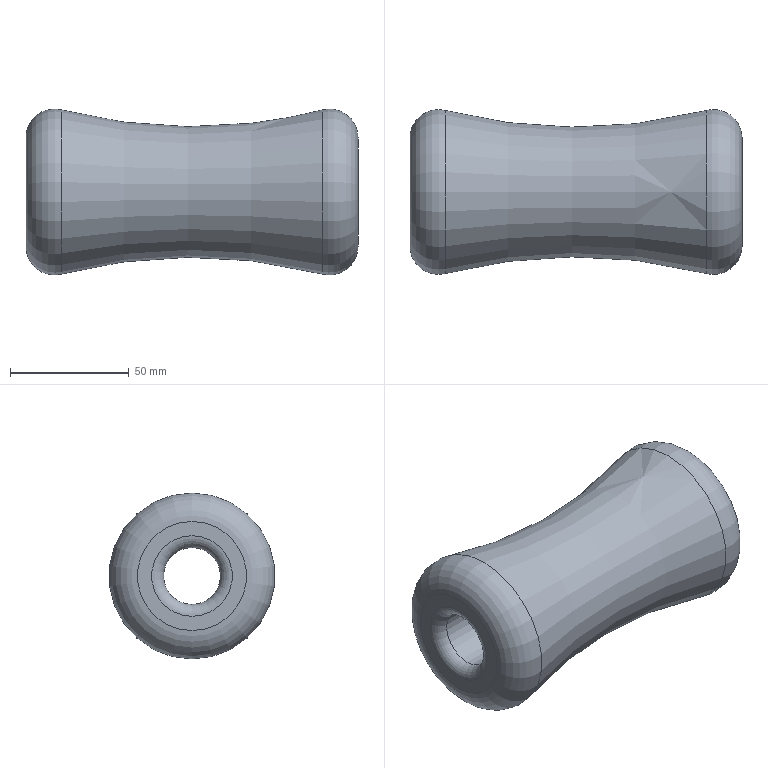Part | STEP file | 6101402W | 1 solid | 8 faces | box 140 x 70 x 70 mm | volume 348651 mm3 | torus 5 | plane 2 | cylinder 1 | commonest cylinder face diameters 24 x1
STEP:
#1=CARTESIAN_POINT('',(0.,0.,0.));
#2=DIRECTION('',(0.,0.,1.));
#3=DIRECTION('',(1.,0.,0.));
#4=AXIS2_PLACEMENT_3D('',#1,#2,#3);
#5=CARTESIAN_POINT('',(70.,0.,17.));
#6=VERTEX_POINT('',#5);
#7=CARTESIAN_POINT('',(70.,0.,0.));
#8=DIRECTION('',(-1.,0.,0.));
#9=DIRECTION('',(0.,0.,1.));
#10=AXIS2_PLACEMENT_3D('',#7,#8,#9);
#11=CIRCLE('',#10,17.);
#12=CARTESIAN_POINT('',(65.,0.,0.));
#13=DIRECTION('',(-1.,0.,0.));
#14=DIRECTION('',(0.,0.,1.));
#15=AXIS2_PLACEMENT_3D('',#12,#13,#14);
#16=TOROIDAL_SURFACE('',#15,17.,5.);
#17=CARTESIAN_POINT('',(0.,4.712));
#18=DIRECTION('',(1.,0.));
#19=VECTOR('',#18,1.);
#20=LINE('',#17,#19);
#21=(GEOMETRIC_REPRESENTATION_CONTEXT(2)PARAMETRIC_REPRESENTATION_CONTEXT()REPRESENTATION_CONTEXT('',''));
#22=DEFINITIONAL_REPRESENTATION('',(#20),#21);
#23=PCURVE('',#16,#22);
#24=CARTESIAN_POINT('',(70.,23.,0.));
#25=DIRECTION('',(-1.,0.,0.));
#26=DIRECTION('',(0.,0.,1.));
#27=AXIS2_PLACEMENT_3D('',#24,#25,#26);
#28=PLANE('',#27);
#29=CARTESIAN_POINT('',(0.,-23.));
#30=DIRECTION('',(1.,0.));
#31=AXIS2_PLACEMENT_2D('',#29,#30);
#32=CIRCLE('',#31,17.);
#33=(GEOMETRIC_REPRESENTATION_CONTEXT(2)PARAMETRIC_REPRESENTATION_CONTEXT()REPRESENTATION_CONTEXT('',''));
#34=DEFINITIONAL_REPRESENTATION('',(#32),#33);
#35=PCURVE('',#28,#34);
#36=SURFACE_CURVE('',#11,(#23,#35),.PCURVE_S1.);
#37=EDGE_CURVE('',#6,#6,#36,.T.);
#38=ORIENTED_EDGE('',*,*,#37,.F.);
#39=CARTESIAN_POINT('',(65.,0.,12.));
#40=VERTEX_POINT('',#39);
#41=CARTESIAN_POINT('',(65.,0.,12.));
#42=CARTESIAN_POINT('',(66.337,0.,12.));
#43=CARTESIAN_POINT('',(67.639,0.,12.425));
#44=CARTESIAN_POINT('',(68.76,0.,13.24));
#45=CARTESIAN_POINT('',(69.575,0.,14.361));
#46=CARTESIAN_POINT('',(70.,0.,15.663));
#47=CARTESIAN_POINT('',(70.,0.,17.));
#48=(BOUNDED_CURVE()B_SPLINE_CURVE(6,(#41,#42,#43,#44,#45,#46,#47),.UNSPECIFIED.,.F.,.F.)B_SPLINE_CURVE_WITH_KNOTS((7,7),(3.142,4.712),.PIECEWISE_BEZIER_KNOTS.)CURVE()GEOMETRIC_REPRESENTATION_ITEM()RATIONAL_B_SPLINE_CURVE((1.031,1.01,0.9979,0.994,0.9979,1.01,1.031))REPRESENTATION_ITEM(''));
#49=CARTESIAN_POINT('',(0.,0.));
#50=DIRECTION('',(0.,1.));
#51=VECTOR('',#50,1.);
#52=LINE('',#49,#51);
#53=(GEOMETRIC_REPRESENTATION_CONTEXT(2)PARAMETRIC_REPRESENTATION_CONTEXT()REPRESENTATION_CONTEXT('',''));
#54=DEFINITIONAL_REPRESENTATION('',(#52),#53);
#55=PCURVE('',#16,#54);
#56=CARTESIAN_POINT('',(6.283,0.));
#57=DIRECTION('',(0.,1.));
#58=VECTOR('',#57,1.);
#59=LINE('',#56,#58);
#60=(GEOMETRIC_REPRESENTATION_CONTEXT(2)PARAMETRIC_REPRESENTATION_CONTEXT()REPRESENTATION_CONTEXT('',''));
#61=DEFINITIONAL_REPRESENTATION('',(#59),#60);
#62=PCURVE('',#16,#61);
#63=SEAM_CURVE('',#48,(#55,#62),.PCURVE_S1.);
#64=EDGE_CURVE('',#40,#6,#63,.T.);
#65=ORIENTED_EDGE('',*,*,#64,.F.);
#66=CARTESIAN_POINT('',(65.,0.,0.));
#67=DIRECTION('',(-1.,0.,0.));
#68=DIRECTION('',(0.,0.,1.));
#69=AXIS2_PLACEMENT_3D('',#66,#67,#68);
#70=CIRCLE('',#69,12.);
#71=CARTESIAN_POINT('',(0.,3.142));
#72=DIRECTION('',(1.,0.));
#73=VECTOR('',#72,1.);
#74=LINE('',#71,#73);
#75=(GEOMETRIC_REPRESENTATION_CONTEXT(2)PARAMETRIC_REPRESENTATION_CONTEXT()REPRESENTATION_CONTEXT('',''));
#76=DEFINITIONAL_REPRESENTATION('',(#74),#75);
#77=PCURVE('',#16,#76);
#78=CARTESIAN_POINT('',(-73.428,0.,0.));
#79=DIRECTION('',(-1.,0.,0.));
#80=DIRECTION('',(0.,0.,1.));
#81=AXIS2_PLACEMENT_3D('',#78,#79,#80);
#82=CYLINDRICAL_SURFACE('',#81,12.);
#83=CARTESIAN_POINT('',(0.,-138.428));
#84=DIRECTION('',(1.,0.));
#85=VECTOR('',#84,1.);
#86=LINE('',#83,#85);
#87=(GEOMETRIC_REPRESENTATION_CONTEXT(2)PARAMETRIC_REPRESENTATION_CONTEXT()REPRESENTATION_CONTEXT('',''));
#88=DEFINITIONAL_REPRESENTATION('',(#86),#87);
#89=PCURVE('',#82,#88);
#90=SURFACE_CURVE('',#70,(#77,#89),.PCURVE_S1.);
#91=EDGE_CURVE('',#40,#40,#90,.T.);
#92=ORIENTED_EDGE('',*,*,#91,.T.);
#93=ORIENTED_EDGE('',*,*,#64,.T.);
#94=EDGE_LOOP('',(#38,#65,#92,#93));
#95=FACE_BOUND('',#94,.T.);
#96=ADVANCED_FACE('',(#95),#16,.T.);
#97=CARTESIAN_POINT('',(70.,0.,23.));
#98=VERTEX_POINT('',#97);
#99=CARTESIAN_POINT('',(70.,0.,0.));
#100=DIRECTION('',(-1.,0.,0.));
#101=DIRECTION('',(0.,0.,1.));
#102=AXIS2_PLACEMENT_3D('',#99,#100,#101);
#103=CIRCLE('',#102,23.);
#104=CARTESIAN_POINT('',(0.,-23.));
#105=DIRECTION('',(1.,0.));
#106=AXIS2_PLACEMENT_2D('',#104,#105);
#107=CIRCLE('',#106,23.);
#108=(GEOMETRIC_REPRESENTATION_CONTEXT(2)PARAMETRIC_REPRESENTATION_CONTEXT()REPRESENTATION_CONTEXT('',''));
#109=DEFINITIONAL_REPRESENTATION('',(#107),#108);
#110=PCURVE('',#28,#109);
#111=CARTESIAN_POINT('',(58.,0.,0.));
#112=DIRECTION('',(-1.,0.,0.));
#113=DIRECTION('',(0.,0.,1.));
#114=AXIS2_PLACEMENT_3D('',#111,#112,#113);
#115=TOROIDAL_SURFACE('',#114,23.,12.);
#116=CARTESIAN_POINT('',(0.,4.712));
#117=DIRECTION('',(1.,0.));
#118=VECTOR('',#117,1.);
#119=LINE('',#116,#118);
#120=(GEOMETRIC_REPRESENTATION_CONTEXT(2)PARAMETRIC_REPRESENTATION_CONTEXT()REPRESENTATION_CONTEXT('',''));
#121=DEFINITIONAL_REPRESENTATION('',(#119),#120);
#122=PCURVE('',#115,#121);
#123=SURFACE_CURVE('',#103,(#110,#122),.PCURVE_S1.);
#124=EDGE_CURVE('',#98,#98,#123,.T.);
#125=ORIENTED_EDGE('',*,*,#124,.F.);
#126=EDGE_LOOP('',(#125));
#127=FACE_BOUND('',#126,.T.);
#128=ORIENTED_EDGE('',*,*,#37,.T.);
#129=EDGE_LOOP('',(#128));
#130=FACE_BOUND('',#129,.T.);
#131=ADVANCED_FACE('',(#127,#130),#28,.F.);
#132=CARTESIAN_POINT('',(54.963,0.,34.609));
#133=VERTEX_POINT('',#132);
#134=CARTESIAN_POINT('',(54.963,0.,0.));
#135=DIRECTION('',(-1.,0.,0.));
#136=DIRECTION('',(0.,0.,1.));
#137=AXIS2_PLACEMENT_3D('',#134,#135,#136);
#138=CIRCLE('',#137,34.609);
#139=CARTESIAN_POINT('',(0.,6.539));
#140=DIRECTION('',(1.,0.));
#141=VECTOR('',#140,1.);
#142=LINE('',#139,#141);
#143=(GEOMETRIC_REPRESENTATION_CONTEXT(2)PARAMETRIC_REPRESENTATION_CONTEXT()REPRESENTATION_CONTEXT('',''));
#144=DEFINITIONAL_REPRESENTATION('',(#142),#143);
#145=PCURVE('',#115,#144);
#146=CARTESIAN_POINT('',(0.,0.,0.));
#147=DIRECTION('',(-1.,0.,0.));
#148=DIRECTION('',(0.,0.,1.));
#149=AXIS2_PLACEMENT_3D('',#146,#147,#148);
#150=TOROIDAL_SURFACE('',#149,244.698,217.16);
#151=CARTESIAN_POINT('',(0.,3.397));
#152=DIRECTION('',(1.,0.));
#153=VECTOR('',#152,1.);
#154=LINE('',#151,#153);
#155=(GEOMETRIC_REPRESENTATION_CONTEXT(2)PARAMETRIC_REPRESENTATION_CONTEXT()REPRESENTATION_CONTEXT('',''));
#156=DEFINITIONAL_REPRESENTATION('',(#154),#155);
#157=PCURVE('',#150,#156);
#158=SURFACE_CURVE('',#138,(#145,#157),.PCURVE_S1.);
#159=EDGE_CURVE('',#133,#133,#158,.T.);
#160=ORIENTED_EDGE('',*,*,#159,.F.);
#161=CARTESIAN_POINT('',(70.,0.,23.));
#162=CARTESIAN_POINT('',(70.,0.,26.131));
#163=CARTESIAN_POINT('',(69.047,0.,29.263));
#164=CARTESIAN_POINT('',(67.14,0.,32.046));
#165=CARTESIAN_POINT('',(64.438,0.,34.132));
#166=CARTESIAN_POINT('',(61.263,0.,35.272));
#167=CARTESIAN_POINT('',(57.992,0.,35.402));
#168=CARTESIAN_POINT('',(54.963,0.,34.609));
#169=B_SPLINE_CURVE_WITH_KNOTS('',7,(#161,#162,#163,#164,#165,#166,#167,#168),.UNSPECIFIED.,.F.,.F.,(8,8),(-1.571,0.2559),.PIECEWISE_BEZIER_KNOTS.);
#170=CARTESIAN_POINT('',(0.,6.283));
#171=DIRECTION('',(0.,1.));
#172=VECTOR('',#171,1.);
#173=LINE('',#170,#172);
#174=(GEOMETRIC_REPRESENTATION_CONTEXT(2)PARAMETRIC_REPRESENTATION_CONTEXT()REPRESENTATION_CONTEXT('',''));
#175=DEFINITIONAL_REPRESENTATION('',(#173),#174);
#176=PCURVE('',#115,#175);
#177=CARTESIAN_POINT('',(6.283,6.283));
#178=DIRECTION('',(0.,1.));
#179=VECTOR('',#178,1.);
#180=LINE('',#177,#179);
#181=(GEOMETRIC_REPRESENTATION_CONTEXT(2)PARAMETRIC_REPRESENTATION_CONTEXT()REPRESENTATION_CONTEXT('',''));
#182=DEFINITIONAL_REPRESENTATION('',(#180),#181);
#183=PCURVE('',#115,#182);
#184=SEAM_CURVE('',#169,(#176,#183),.PCURVE_S1.);
#185=EDGE_CURVE('',#98,#133,#184,.T.);
#186=ORIENTED_EDGE('',*,*,#185,.F.);
#187=ORIENTED_EDGE('',*,*,#124,.T.);
#188=ORIENTED_EDGE('',*,*,#185,.T.);
#189=EDGE_LOOP('',(#160,#186,#187,#188));
#190=FACE_BOUND('',#189,.T.);
#191=ADVANCED_FACE('',(#190),#115,.T.);
#192=CARTESIAN_POINT('',(-54.963,0.,34.609));
#193=VERTEX_POINT('',#192);
#194=CARTESIAN_POINT('',(-54.963,0.,0.));
#195=DIRECTION('',(-1.,0.,0.));
#196=DIRECTION('',(0.,0.,1.));
#197=AXIS2_PLACEMENT_3D('',#194,#195,#196);
#198=CIRCLE('',#197,34.609);
#199=CARTESIAN_POINT('',(0.,2.886));
#200=DIRECTION('',(1.,0.));
#201=VECTOR('',#200,1.);
#202=LINE('',#199,#201);
#203=(GEOMETRIC_REPRESENTATION_CONTEXT(2)PARAMETRIC_REPRESENTATION_CONTEXT()REPRESENTATION_CONTEXT('',''));
#204=DEFINITIONAL_REPRESENTATION('',(#202),#203);
#205=PCURVE('',#150,#204);
#206=CARTESIAN_POINT('',(-58.,0.,0.));
#207=DIRECTION('',(-1.,0.,0.));
#208=DIRECTION('',(0.,0.,1.));
#209=AXIS2_PLACEMENT_3D('',#206,#207,#208);
#210=TOROIDAL_SURFACE('',#209,23.,12.);
#211=CARTESIAN_POINT('',(0.,6.027));
#212=DIRECTION('',(1.,0.));
#213=VECTOR('',#212,1.);
#214=LINE('',#211,#213);
#215=(GEOMETRIC_REPRESENTATION_CONTEXT(2)PARAMETRIC_REPRESENTATION_CONTEXT()REPRESENTATION_CONTEXT('',''));
#216=DEFINITIONAL_REPRESENTATION('',(#214),#215);
#217=PCURVE('',#210,#216);
#218=SURFACE_CURVE('',#198,(#205,#217),.PCURVE_S1.);
#219=EDGE_CURVE('',#193,#193,#218,.T.);
#220=ORIENTED_EDGE('',*,*,#219,.T.);
#221=CARTESIAN_POINT('',(-54.963,0.,34.609));
#222=CARTESIAN_POINT('',(-37.004,0.,29.911));
#223=CARTESIAN_POINT('',(-18.612,0.,27.066));
#224=CARTESIAN_POINT('',(0.,0.,26.113));
#225=CARTESIAN_POINT('',(18.612,0.,27.066));
#226=CARTESIAN_POINT('',(37.004,0.,29.911));
#227=CARTESIAN_POINT('',(54.963,0.,34.609));
#228=(BOUNDED_CURVE()B_SPLINE_CURVE(6,(#221,#222,#223,#224,#225,#226,#227),.UNSPECIFIED.,.F.,.F.)B_SPLINE_CURVE_WITH_KNOTS((7,7),(2.886,3.397),.PIECEWISE_BEZIER_KNOTS.)CURVE()GEOMETRIC_REPRESENTATION_ITEM()RATIONAL_B_SPLINE_CURVE((1.003,1.001,0.9998,0.9993,0.9998,1.001,1.003))REPRESENTATION_ITEM(''));
#229=CARTESIAN_POINT('',(6.283,0.));
#230=DIRECTION('',(0.,1.));
#231=VECTOR('',#230,1.);
#232=LINE('',#229,#231);
#233=(GEOMETRIC_REPRESENTATION_CONTEXT(2)PARAMETRIC_REPRESENTATION_CONTEXT()REPRESENTATION_CONTEXT('',''));
#234=DEFINITIONAL_REPRESENTATION('',(#232),#233);
#235=PCURVE('',#150,#234);
#236=CARTESIAN_POINT('',(0.,0.));
#237=DIRECTION('',(0.,1.));
#238=VECTOR('',#237,1.);
#239=LINE('',#236,#238);
#240=(GEOMETRIC_REPRESENTATION_CONTEXT(2)PARAMETRIC_REPRESENTATION_CONTEXT()REPRESENTATION_CONTEXT('',''));
#241=DEFINITIONAL_REPRESENTATION('',(#239),#240);
#242=PCURVE('',#150,#241);
#243=SEAM_CURVE('',#228,(#235,#242),.PCURVE_S1.);
#244=EDGE_CURVE('',#193,#133,#243,.T.);
#245=ORIENTED_EDGE('',*,*,#244,.T.);
#246=ORIENTED_EDGE('',*,*,#159,.F.);
#247=ORIENTED_EDGE('',*,*,#244,.F.);
#248=EDGE_LOOP('',(#220,#245,#246,#247));
#249=FACE_BOUND('',#248,.F.);
#250=ADVANCED_FACE('',(#249),#150,.F.);
#251=CARTESIAN_POINT('',(-70.,0.,23.));
#252=VERTEX_POINT('',#251);
#253=CARTESIAN_POINT('',(-70.,0.,0.));
#254=DIRECTION('',(-1.,0.,0.));
#255=DIRECTION('',(0.,0.,1.));
#256=AXIS2_PLACEMENT_3D('',#253,#254,#255);
#257=CIRCLE('',#256,23.);
#258=CARTESIAN_POINT('',(0.,7.854));
#259=DIRECTION('',(1.,0.));
#260=VECTOR('',#259,1.);
#261=LINE('',#258,#260);
#262=(GEOMETRIC_REPRESENTATION_CONTEXT(2)PARAMETRIC_REPRESENTATION_CONTEXT()REPRESENTATION_CONTEXT('',''));
#263=DEFINITIONAL_REPRESENTATION('',(#261),#262);
#264=PCURVE('',#210,#263);
#265=CARTESIAN_POINT('',(-70.,23.,0.));
#266=DIRECTION('',(1.,0.,0.));
#267=DIRECTION('',(0.,0.,-1.));
#268=AXIS2_PLACEMENT_3D('',#265,#266,#267);
#269=PLANE('',#268);
#270=CARTESIAN_POINT('',(-23.,-23.));
#271=CARTESIAN_POINT('',(-23.,16.837));
#272=CARTESIAN_POINT('',(11.5,-3.081));
#273=CARTESIAN_POINT('',(46.,-23.));
#274=CARTESIAN_POINT('',(11.5,-42.919));
#275=CARTESIAN_POINT('',(-23.,-62.837));
#276=CARTESIAN_POINT('',(-23.,-23.));
#277=(BOUNDED_CURVE()B_SPLINE_CURVE(2,(#270,#271,#272,#273,#274,#275,#276),.UNSPECIFIED.,.T.,.F.)B_SPLINE_CURVE_WITH_KNOTS((1,2,2,2,2,1),(-2.094,0.,2.094,4.189,6.283,8.378),.UNSPECIFIED.)CURVE()GEOMETRIC_REPRESENTATION_ITEM()RATIONAL_B_SPLINE_CURVE((1.,0.5,1.,0.5,1.,0.5,1.))REPRESENTATION_ITEM(''));
#278=(GEOMETRIC_REPRESENTATION_CONTEXT(2)PARAMETRIC_REPRESENTATION_CONTEXT()REPRESENTATION_CONTEXT('',''));
#279=DEFINITIONAL_REPRESENTATION('',(#277),#278);
#280=PCURVE('',#269,#279);
#281=SURFACE_CURVE('',#257,(#264,#280),.PCURVE_S1.);
#282=EDGE_CURVE('',#252,#252,#281,.T.);
#283=ORIENTED_EDGE('',*,*,#282,.F.);
#284=CARTESIAN_POINT('',(-54.963,0.,34.609));
#285=CARTESIAN_POINT('',(-57.992,0.,35.402));
#286=CARTESIAN_POINT('',(-61.263,0.,35.272));
#287=CARTESIAN_POINT('',(-64.438,0.,34.132));
#288=CARTESIAN_POINT('',(-67.14,0.,32.046));
#289=CARTESIAN_POINT('',(-69.047,0.,29.263));
#290=CARTESIAN_POINT('',(-70.,0.,26.131));
#291=CARTESIAN_POINT('',(-70.,0.,23.));
#292=B_SPLINE_CURVE_WITH_KNOTS('',7,(#284,#285,#286,#287,#288,#289,#290,#291),.UNSPECIFIED.,.F.,.F.,(8,8),(-0.2559,1.571),.PIECEWISE_BEZIER_KNOTS.);
#293=CARTESIAN_POINT('',(0.,6.283));
#294=DIRECTION('',(0.,1.));
#295=VECTOR('',#294,1.);
#296=LINE('',#293,#295);
#297=(GEOMETRIC_REPRESENTATION_CONTEXT(2)PARAMETRIC_REPRESENTATION_CONTEXT()REPRESENTATION_CONTEXT('',''));
#298=DEFINITIONAL_REPRESENTATION('',(#296),#297);
#299=PCURVE('',#210,#298);
#300=CARTESIAN_POINT('',(6.283,6.283));
#301=DIRECTION('',(0.,1.));
#302=VECTOR('',#301,1.);
#303=LINE('',#300,#302);
#304=(GEOMETRIC_REPRESENTATION_CONTEXT(2)PARAMETRIC_REPRESENTATION_CONTEXT()REPRESENTATION_CONTEXT('',''));
#305=DEFINITIONAL_REPRESENTATION('',(#303),#304);
#306=PCURVE('',#210,#305);
#307=SEAM_CURVE('',#292,(#299,#306),.PCURVE_S1.);
#308=EDGE_CURVE('',#193,#252,#307,.T.);
#309=ORIENTED_EDGE('',*,*,#308,.F.);
#310=ORIENTED_EDGE('',*,*,#219,.T.);
#311=ORIENTED_EDGE('',*,*,#308,.T.);
#312=EDGE_LOOP('',(#283,#309,#310,#311));
#313=FACE_BOUND('',#312,.T.);
#314=ADVANCED_FACE('',(#313),#210,.T.);
#315=CARTESIAN_POINT('',(-70.,0.,17.));
#316=VERTEX_POINT('',#315);
#317=CARTESIAN_POINT('',(-70.,0.,0.));
#318=DIRECTION('',(-1.,0.,0.));
#319=DIRECTION('',(0.,0.,1.));
#320=AXIS2_PLACEMENT_3D('',#317,#318,#319);
#321=CIRCLE('',#320,17.);
#322=CARTESIAN_POINT('',(-17.,-23.));
#323=CARTESIAN_POINT('',(-17.,6.445));
#324=CARTESIAN_POINT('',(8.5,-8.278));
#325=CARTESIAN_POINT('',(34.,-23.));
#326=CARTESIAN_POINT('',(8.5,-37.722));
#327=CARTESIAN_POINT('',(-17.,-52.445));
#328=CARTESIAN_POINT('',(-17.,-23.));
#329=(BOUNDED_CURVE()B_SPLINE_CURVE(2,(#322,#323,#324,#325,#326,#327,#328),.UNSPECIFIED.,.T.,.F.)B_SPLINE_CURVE_WITH_KNOTS((1,2,2,2,2,1),(-2.094,0.,2.094,4.189,6.283,8.378),.UNSPECIFIED.)CURVE()GEOMETRIC_REPRESENTATION_ITEM()RATIONAL_B_SPLINE_CURVE((1.,0.5,1.,0.5,1.,0.5,1.))REPRESENTATION_ITEM(''));
#330=(GEOMETRIC_REPRESENTATION_CONTEXT(2)PARAMETRIC_REPRESENTATION_CONTEXT()REPRESENTATION_CONTEXT('',''));
#331=DEFINITIONAL_REPRESENTATION('',(#329),#330);
#332=PCURVE('',#269,#331);
#333=CARTESIAN_POINT('',(-65.,0.,0.));
#334=DIRECTION('',(-1.,0.,0.));
#335=DIRECTION('',(0.,0.,1.));
#336=AXIS2_PLACEMENT_3D('',#333,#334,#335);
#337=TOROIDAL_SURFACE('',#336,17.,5.);
#338=CARTESIAN_POINT('',(0.,7.854));
#339=DIRECTION('',(1.,0.));
#340=VECTOR('',#339,1.);
#341=LINE('',#338,#340);
#342=(GEOMETRIC_REPRESENTATION_CONTEXT(2)PARAMETRIC_REPRESENTATION_CONTEXT()REPRESENTATION_CONTEXT('',''));
#343=DEFINITIONAL_REPRESENTATION('',(#341),#342);
#344=PCURVE('',#337,#343);
#345=SURFACE_CURVE('',#321,(#332,#344),.PCURVE_S1.);
#346=EDGE_CURVE('',#316,#316,#345,.T.);
#347=ORIENTED_EDGE('',*,*,#346,.F.);
#348=EDGE_LOOP('',(#347));
#349=FACE_BOUND('',#348,.T.);
#350=ORIENTED_EDGE('',*,*,#282,.T.);
#351=EDGE_LOOP('',(#350));
#352=FACE_BOUND('',#351,.T.);
#353=ADVANCED_FACE('',(#349,#352),#269,.F.);
#354=CARTESIAN_POINT('',(-65.,0.,12.));
#355=VERTEX_POINT('',#354);
#356=CARTESIAN_POINT('',(-65.,0.,0.));
#357=DIRECTION('',(-1.,0.,0.));
#358=DIRECTION('',(0.,0.,1.));
#359=AXIS2_PLACEMENT_3D('',#356,#357,#358);
#360=CIRCLE('',#359,12.);
#361=CARTESIAN_POINT('',(0.,9.425));
#362=DIRECTION('',(1.,0.));
#363=VECTOR('',#362,1.);
#364=LINE('',#361,#363);
#365=(GEOMETRIC_REPRESENTATION_CONTEXT(2)PARAMETRIC_REPRESENTATION_CONTEXT()REPRESENTATION_CONTEXT('',''));
#366=DEFINITIONAL_REPRESENTATION('',(#364),#365);
#367=PCURVE('',#337,#366);
#368=CARTESIAN_POINT('',(0.,-8.428));
#369=DIRECTION('',(1.,0.));
#370=VECTOR('',#369,1.);
#371=LINE('',#368,#370);
#372=(GEOMETRIC_REPRESENTATION_CONTEXT(2)PARAMETRIC_REPRESENTATION_CONTEXT()REPRESENTATION_CONTEXT('',''));
#373=DEFINITIONAL_REPRESENTATION('',(#371),#372);
#374=PCURVE('',#82,#373);
#375=SURFACE_CURVE('',#360,(#367,#374),.PCURVE_S1.);
#376=EDGE_CURVE('',#355,#355,#375,.T.);
#377=ORIENTED_EDGE('',*,*,#376,.F.);
#378=CARTESIAN_POINT('',(-70.,0.,17.));
#379=CARTESIAN_POINT('',(-70.,0.,15.663));
#380=CARTESIAN_POINT('',(-69.575,0.,14.361));
#381=CARTESIAN_POINT('',(-68.76,0.,13.24));
#382=CARTESIAN_POINT('',(-67.639,0.,12.425));
#383=CARTESIAN_POINT('',(-66.337,0.,12.));
#384=CARTESIAN_POINT('',(-65.,0.,12.));
#385=(BOUNDED_CURVE()B_SPLINE_CURVE(6,(#378,#379,#380,#381,#382,#383,#384),.UNSPECIFIED.,.F.,.F.)B_SPLINE_CURVE_WITH_KNOTS((7,7),(1.571,3.142),.PIECEWISE_BEZIER_KNOTS.)CURVE()GEOMETRIC_REPRESENTATION_ITEM()RATIONAL_B_SPLINE_CURVE((1.031,1.01,0.9979,0.994,0.9979,1.01,1.031))REPRESENTATION_ITEM(''));
#386=CARTESIAN_POINT('',(0.,6.283));
#387=DIRECTION('',(0.,1.));
#388=VECTOR('',#387,1.);
#389=LINE('',#386,#388);
#390=(GEOMETRIC_REPRESENTATION_CONTEXT(2)PARAMETRIC_REPRESENTATION_CONTEXT()REPRESENTATION_CONTEXT('',''));
#391=DEFINITIONAL_REPRESENTATION('',(#389),#390);
#392=PCURVE('',#337,#391);
#393=CARTESIAN_POINT('',(6.283,6.283));
#394=DIRECTION('',(0.,1.));
#395=VECTOR('',#394,1.);
#396=LINE('',#393,#395);
#397=(GEOMETRIC_REPRESENTATION_CONTEXT(2)PARAMETRIC_REPRESENTATION_CONTEXT()REPRESENTATION_CONTEXT('',''));
#398=DEFINITIONAL_REPRESENTATION('',(#396),#397);
#399=PCURVE('',#337,#398);
#400=SEAM_CURVE('',#385,(#392,#399),.PCURVE_S1.);
#401=EDGE_CURVE('',#316,#355,#400,.T.);
#402=ORIENTED_EDGE('',*,*,#401,.F.);
#403=ORIENTED_EDGE('',*,*,#346,.T.);
#404=ORIENTED_EDGE('',*,*,#401,.T.);
#405=EDGE_LOOP('',(#377,#402,#403,#404));
#406=FACE_BOUND('',#405,.T.);
#407=ADVANCED_FACE('',(#406),#337,.T.);
#408=ORIENTED_EDGE('',*,*,#91,.T.);
#409=CARTESIAN_POINT('',(65.,0.,12.));
#410=CARTESIAN_POINT('',(-65.,0.,12.));
#411=B_SPLINE_CURVE_WITH_KNOTS('',1,(#409,#410),.UNSPECIFIED.,.F.,.F.,(2,2),(-138.428,-8.428),.PIECEWISE_BEZIER_KNOTS.);
#412=CARTESIAN_POINT('',(6.283,0.));
#413=DIRECTION('',(0.,1.));
#414=VECTOR('',#413,1.);
#415=LINE('',#412,#414);
#416=(GEOMETRIC_REPRESENTATION_CONTEXT(2)PARAMETRIC_REPRESENTATION_CONTEXT()REPRESENTATION_CONTEXT('',''));
#417=DEFINITIONAL_REPRESENTATION('',(#415),#416);
#418=PCURVE('',#82,#417);
#419=CARTESIAN_POINT('',(0.,0.));
#420=DIRECTION('',(0.,1.));
#421=VECTOR('',#420,1.);
#422=LINE('',#419,#421);
#423=(GEOMETRIC_REPRESENTATION_CONTEXT(2)PARAMETRIC_REPRESENTATION_CONTEXT()REPRESENTATION_CONTEXT('',''));
#424=DEFINITIONAL_REPRESENTATION('',(#422),#423);
#425=PCURVE('',#82,#424);
#426=SEAM_CURVE('',#411,(#418,#425),.PCURVE_S1.);
#427=EDGE_CURVE('',#40,#355,#426,.T.);
#428=ORIENTED_EDGE('',*,*,#427,.T.);
#429=ORIENTED_EDGE('',*,*,#376,.F.);
#430=ORIENTED_EDGE('',*,*,#427,.F.);
#431=EDGE_LOOP('',(#408,#428,#429,#430));
#432=FACE_BOUND('',#431,.F.);
#433=ADVANCED_FACE('',(#432),#82,.F.);
#434=CLOSED_SHELL('',(#96,#131,#191,#250,#314,#353,#407,#433));
#435=MANIFOLD_SOLID_BREP('',#434);
#436=(LENGTH_UNIT()NAMED_UNIT(*)SI_UNIT(.MILLI.,.METRE.));
#437=UNCERTAINTY_MEASURE_WITH_UNIT(LENGTH_MEASURE(0.00001),#436,'','');
#438=(NAMED_UNIT(*)PLANE_ANGLE_UNIT()SI_UNIT($,.RADIAN.));
#439=(NAMED_UNIT(*)SI_UNIT($,.STERADIAN.)SOLID_ANGLE_UNIT());
#440=(GEOMETRIC_REPRESENTATION_CONTEXT(3)GLOBAL_UNCERTAINTY_ASSIGNED_CONTEXT((#437))GLOBAL_UNIT_ASSIGNED_CONTEXT((#436,#438,#439))REPRESENTATION_CONTEXT('',''));
#441=ADVANCED_BREP_SHAPE_REPRESENTATION('',(#4,#435),#440);